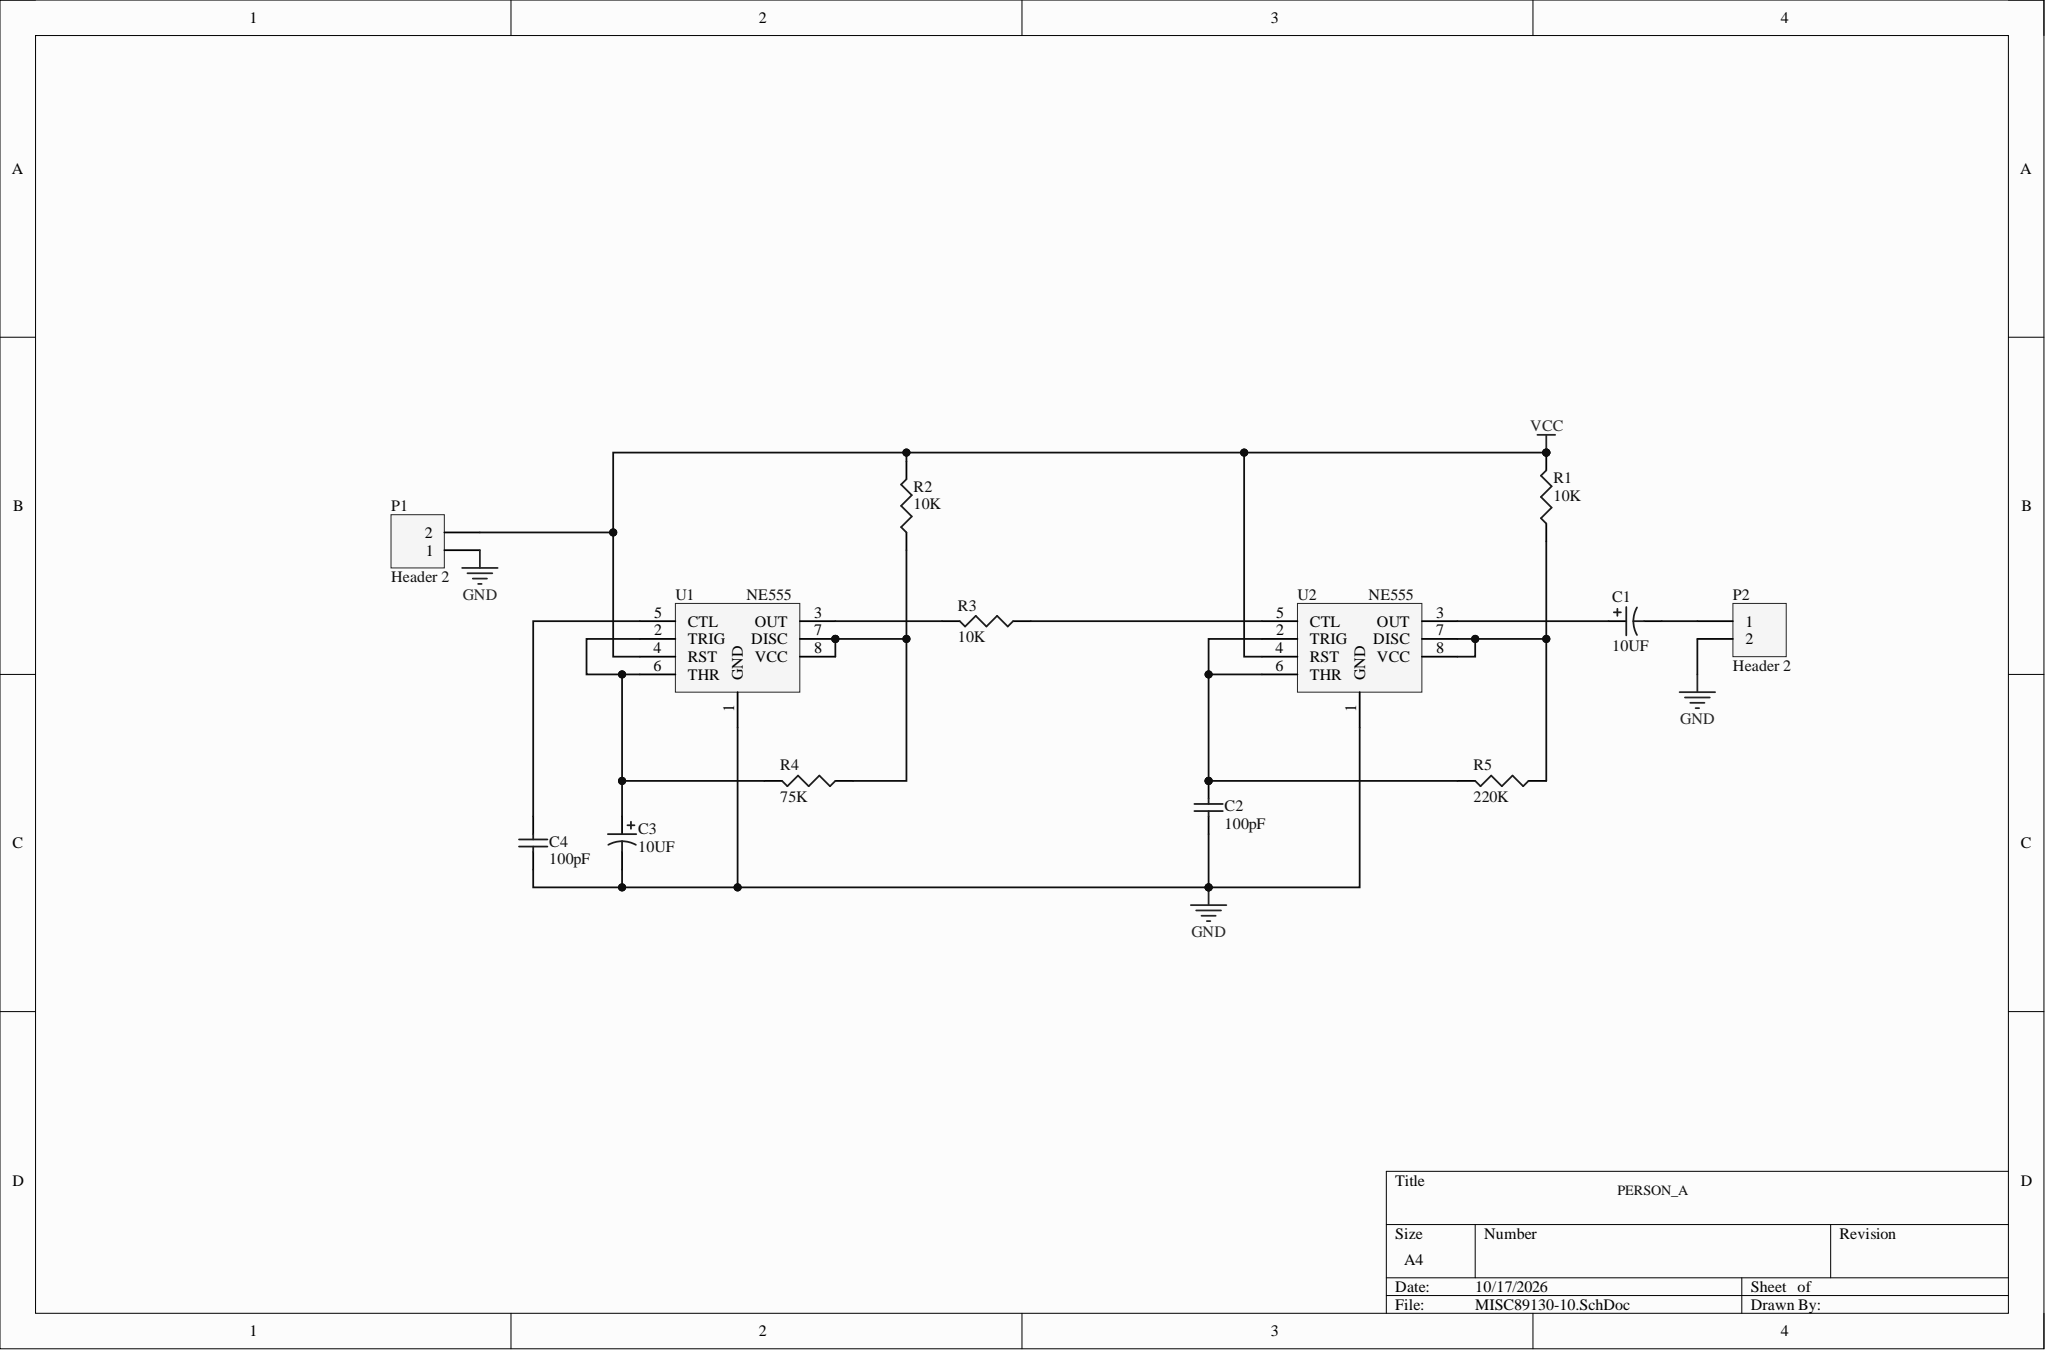Circuit board | Altium Designer | 13 parts | 11 nets
Bill of materials:
Comment,Description,Designator,Footprint,LibRef,Quantity
"10UF","Polarized Capacitor (Surface Mount)","C1, C3","C1206","Cap Pol3","2"
"Cap","Capacitor","C2, C4","J1-0603","Cap","2"
"Header 2","Header, 2-Pin","P1, P2","HDR1X2","Header 2","2"
"10K","Resistor","R1, R2, R3","J1-0603","Res3","3"
"75K","Resistor","R4","J1-0603","Res3","1"
"220K","Resistor","R5","J1-0603","Res3","1"
"NE555","","U1, U2","DIP8","NE555","2"
Netlist (Protel format):
[
C1
C1206
10UF



]
[
C2
J1-0603
Cap



]
[
C3
C1206
10UF



]
[
C4
J1-0603
Cap



]
[
P1
HDR1X2
Header 2



]
[
P2
HDR1X2
Header 2



]
[
R1
J1-0603
10K



]
[
R2
J1-0603
10K



]
[
R3
J1-0603
10K



]
[
R4
J1-0603
75K



]
[
R5
J1-0603
220K



]
[
U1
DIP8
NE555



]
[
U2
DIP8
NE555



]
(
VCC
P1-2
R1-2
R2-2
U1-4
U2-4
)
(
NetR3_2
R3-2
U1-3
)
(
NetR3_1
R3-1
U2-5
)
(
NetR2_1
R2-1
R4-1
U1-7
U1-8
)
(
NetR1_1
R1-1
R5-1
U2-7
U2-8
)
(
NetC4_2
C4-2
U1-5
)
(
NetC3_1
C3-1
R4-2
U1-2
U1-6
)
(
NetC2_2
C2-2
R5-2
U2-2
U2-6
)
(
NetC1_2
C1-2
P2-1
)
(
NetC1_1
C1-1
U2-3
)
(
GND
C2-1
C3-2
C4-1
P1-1
P2-2
U1-1
U2-1
)